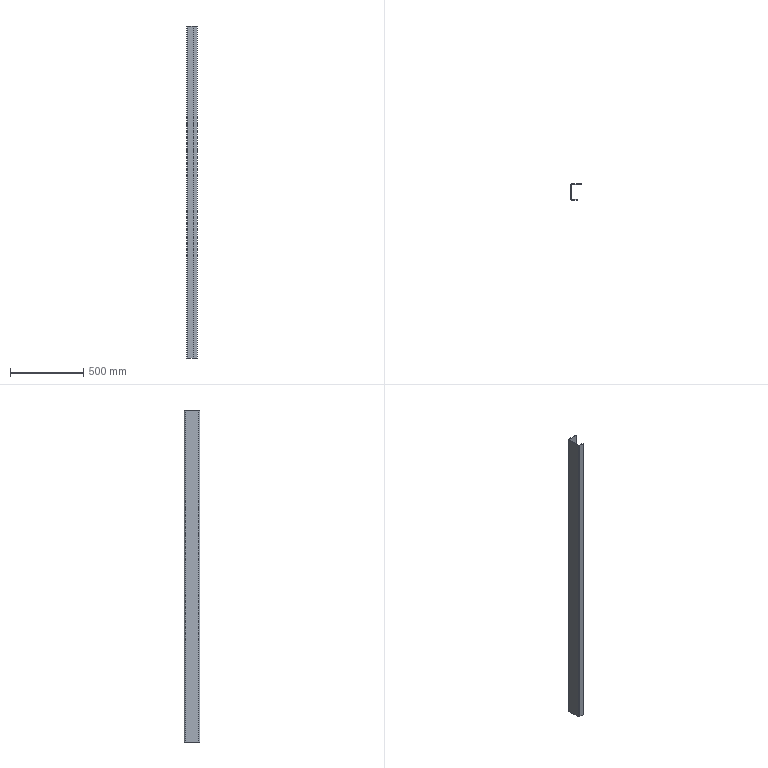Part | STEP file | 750038121 | 1 solid | 14 faces | box 75 x 108 x 2272 mm | volume 1952553 mm3 | plane 10 | cylinder 4 | commonest cylinder face diameters 8 x2 16 x2
STEP:
#1=CARTESIAN_POINT('',(0.,8.,0.));
#2=VERTEX_POINT('',#1);
#3=CARTESIAN_POINT('',(0.,100.,0.));
#4=VERTEX_POINT('',#3);
#5=CARTESIAN_POINT('',(0.,0.,0.));
#6=DIRECTION('',(0.,1.,0.));
#7=VECTOR('',#6,1000.);
#8=LINE('',#5,#7);
#9=EDGE_CURVE('',#2,#4,#8,.T.);
#10=ORIENTED_EDGE('',*,*,#9,.T.);
#11=CARTESIAN_POINT('',(0.,100.,-2272.));
#12=VERTEX_POINT('',#11);
#13=CARTESIAN_POINT('',(0.,100.,0.));
#14=DIRECTION('',(0.,0.,-1.));
#15=VECTOR('',#14,1000.);
#16=LINE('',#13,#15);
#17=EDGE_CURVE('',#4,#12,#16,.T.);
#18=ORIENTED_EDGE('',*,*,#17,.T.);
#19=CARTESIAN_POINT('',(0.,8.,-2272.));
#20=VERTEX_POINT('',#19);
#21=CARTESIAN_POINT('',(0.,0.,-2272.));
#22=DIRECTION('',(0.,-1.,0.));
#23=VECTOR('',#22,1000.);
#24=LINE('',#21,#23);
#25=EDGE_CURVE('',#12,#20,#24,.T.);
#26=ORIENTED_EDGE('',*,*,#25,.T.);
#27=CARTESIAN_POINT('',(0.,8.,0.));
#28=DIRECTION('',(0.,0.,1.));
#29=VECTOR('',#28,1000.);
#30=LINE('',#27,#29);
#31=EDGE_CURVE('',#20,#2,#30,.T.);
#32=ORIENTED_EDGE('',*,*,#31,.T.);
#33=EDGE_LOOP('',(#10,#18,#26,#32));
#34=FACE_OUTER_BOUND('',#33,.T.);
#35=CARTESIAN_POINT('',(0.,0.,0.));
#36=DIRECTION('',(-1.,0.,0.));
#37=DIRECTION('',(0.,0.,1.));
#38=AXIS2_PLACEMENT_3D('',#35,#36,#37);
#39=PLANE('',#38);
#40=ADVANCED_FACE('',(#34),#39,.T.);
#41=CARTESIAN_POINT('',(8.,108.,0.));
#42=VERTEX_POINT('',#41);
#43=CARTESIAN_POINT('',(8.,100.,0.));
#44=DIRECTION('',(0.,0.,-1.));
#45=DIRECTION('',(-1.,0.,0.));
#46=AXIS2_PLACEMENT_3D('',#43,#44,#45);
#47=CIRCLE('',#46,8.);
#48=EDGE_CURVE('',#4,#42,#47,.T.);
#49=ORIENTED_EDGE('',*,*,#48,.T.);
#50=CARTESIAN_POINT('',(8.,108.,-2272.));
#51=VERTEX_POINT('',#50);
#52=CARTESIAN_POINT('',(8.,108.,0.));
#53=DIRECTION('',(0.,0.,-1.));
#54=VECTOR('',#53,1000.);
#55=LINE('',#52,#54);
#56=EDGE_CURVE('',#42,#51,#55,.T.);
#57=ORIENTED_EDGE('',*,*,#56,.T.);
#58=CARTESIAN_POINT('',(8.,100.,-2272.));
#59=DIRECTION('',(0.,0.,1.));
#60=DIRECTION('',(-1.,0.,0.));
#61=AXIS2_PLACEMENT_3D('',#58,#59,#60);
#62=CIRCLE('',#61,8.);
#63=EDGE_CURVE('',#51,#12,#62,.T.);
#64=ORIENTED_EDGE('',*,*,#63,.T.);
#65=ORIENTED_EDGE('',*,*,#17,.F.);
#66=EDGE_LOOP('',(#49,#57,#64,#65));
#67=FACE_OUTER_BOUND('',#66,.T.);
#68=CARTESIAN_POINT('',(8.,100.,0.));
#69=DIRECTION('',(0.,0.,-1.));
#70=DIRECTION('',(-1.,0.,0.));
#71=AXIS2_PLACEMENT_3D('',#68,#69,#70);
#72=CYLINDRICAL_SURFACE('',#71,8.);
#73=ADVANCED_FACE('',(#67),#72,.T.);
#74=CARTESIAN_POINT('',(8.,104.,0.));
#75=VERTEX_POINT('',#74);
#76=CARTESIAN_POINT('',(75.,104.,0.));
#77=VERTEX_POINT('',#76);
#78=CARTESIAN_POINT('',(0.,104.,0.));
#79=DIRECTION('',(1.,0.,0.));
#80=VECTOR('',#79,1000.);
#81=LINE('',#78,#80);
#82=EDGE_CURVE('',#75,#77,#81,.T.);
#83=ORIENTED_EDGE('',*,*,#82,.T.);
#84=CARTESIAN_POINT('',(75.,108.,0.));
#85=VERTEX_POINT('',#84);
#86=CARTESIAN_POINT('',(75.,108.,0.));
#87=DIRECTION('',(0.,1.,0.));
#88=VECTOR('',#87,1000.);
#89=LINE('',#86,#88);
#90=EDGE_CURVE('',#77,#85,#89,.T.);
#91=ORIENTED_EDGE('',*,*,#90,.T.);
#92=CARTESIAN_POINT('',(0.,108.,0.));
#93=DIRECTION('',(-1.,0.,0.));
#94=VECTOR('',#93,1000.);
#95=LINE('',#92,#94);
#96=EDGE_CURVE('',#85,#42,#95,.T.);
#97=ORIENTED_EDGE('',*,*,#96,.T.);
#98=ORIENTED_EDGE('',*,*,#48,.F.);
#99=ORIENTED_EDGE('',*,*,#9,.F.);
#100=CARTESIAN_POINT('',(8.,0.,0.));
#101=VERTEX_POINT('',#100);
#102=CARTESIAN_POINT('',(8.,8.,0.));
#103=DIRECTION('',(0.,0.,1.));
#104=DIRECTION('',(-1.,0.,0.));
#105=AXIS2_PLACEMENT_3D('',#102,#103,#104);
#106=CIRCLE('',#105,8.);
#107=EDGE_CURVE('',#2,#101,#106,.T.);
#108=ORIENTED_EDGE('',*,*,#107,.T.);
#109=CARTESIAN_POINT('',(45.,0.,0.));
#110=VERTEX_POINT('',#109);
#111=CARTESIAN_POINT('',(0.,0.,0.));
#112=DIRECTION('',(1.,0.,0.));
#113=VECTOR('',#112,1000.);
#114=LINE('',#111,#113);
#115=EDGE_CURVE('',#101,#110,#114,.T.);
#116=ORIENTED_EDGE('',*,*,#115,.T.);
#117=CARTESIAN_POINT('',(45.,4.,0.));
#118=VERTEX_POINT('',#117);
#119=CARTESIAN_POINT('',(45.,108.,0.));
#120=DIRECTION('',(0.,1.,0.));
#121=VECTOR('',#120,1000.);
#122=LINE('',#119,#121);
#123=EDGE_CURVE('',#110,#118,#122,.T.);
#124=ORIENTED_EDGE('',*,*,#123,.T.);
#125=CARTESIAN_POINT('',(8.,4.,0.));
#126=VERTEX_POINT('',#125);
#127=CARTESIAN_POINT('',(0.,4.,0.));
#128=DIRECTION('',(-1.,0.,0.));
#129=VECTOR('',#128,1000.);
#130=LINE('',#127,#129);
#131=EDGE_CURVE('',#118,#126,#130,.T.);
#132=ORIENTED_EDGE('',*,*,#131,.T.);
#133=CARTESIAN_POINT('',(4.,8.,0.));
#134=VERTEX_POINT('',#133);
#135=CARTESIAN_POINT('',(8.,8.,0.));
#136=DIRECTION('',(0.,0.,-1.));
#137=DIRECTION('',(-1.,0.,0.));
#138=AXIS2_PLACEMENT_3D('',#135,#136,#137);
#139=CIRCLE('',#138,4.);
#140=EDGE_CURVE('',#126,#134,#139,.T.);
#141=ORIENTED_EDGE('',*,*,#140,.T.);
#142=CARTESIAN_POINT('',(4.,100.,0.));
#143=VERTEX_POINT('',#142);
#144=CARTESIAN_POINT('',(4.,108.,0.));
#145=DIRECTION('',(0.,1.,0.));
#146=VECTOR('',#145,1000.);
#147=LINE('',#144,#146);
#148=EDGE_CURVE('',#134,#143,#147,.T.);
#149=ORIENTED_EDGE('',*,*,#148,.T.);
#150=CARTESIAN_POINT('',(8.,100.,0.));
#151=DIRECTION('',(0.,0.,-1.));
#152=DIRECTION('',(-1.,0.,0.));
#153=AXIS2_PLACEMENT_3D('',#150,#151,#152);
#154=CIRCLE('',#153,4.);
#155=EDGE_CURVE('',#143,#75,#154,.T.);
#156=ORIENTED_EDGE('',*,*,#155,.T.);
#157=EDGE_LOOP('',(#83,#91,#97,#98,#99,#108,#116,#124,#132,#141,#149,#156));
#158=FACE_OUTER_BOUND('',#157,.T.);
#159=CARTESIAN_POINT('',(0.,108.,0.));
#160=DIRECTION('',(0.,0.,1.));
#161=DIRECTION('',(1.,0.,0.));
#162=AXIS2_PLACEMENT_3D('',#159,#160,#161);
#163=PLANE('',#162);
#164=ADVANCED_FACE('',(#158),#163,.T.);
#165=ORIENTED_EDGE('',*,*,#107,.F.);
#166=ORIENTED_EDGE('',*,*,#31,.F.);
#167=CARTESIAN_POINT('',(8.,0.,-2272.));
#168=VERTEX_POINT('',#167);
#169=CARTESIAN_POINT('',(8.,8.,-2272.));
#170=DIRECTION('',(0.,0.,1.));
#171=DIRECTION('',(-1.,0.,0.));
#172=AXIS2_PLACEMENT_3D('',#169,#170,#171);
#173=CIRCLE('',#172,8.);
#174=EDGE_CURVE('',#20,#168,#173,.T.);
#175=ORIENTED_EDGE('',*,*,#174,.T.);
#176=CARTESIAN_POINT('',(8.,0.,0.));
#177=DIRECTION('',(0.,0.,1.));
#178=VECTOR('',#177,1000.);
#179=LINE('',#176,#178);
#180=EDGE_CURVE('',#168,#101,#179,.T.);
#181=ORIENTED_EDGE('',*,*,#180,.T.);
#182=EDGE_LOOP('',(#165,#166,#175,#181));
#183=FACE_OUTER_BOUND('',#182,.T.);
#184=CARTESIAN_POINT('',(8.,8.,0.));
#185=DIRECTION('',(0.,0.,-1.));
#186=DIRECTION('',(-1.,0.,0.));
#187=AXIS2_PLACEMENT_3D('',#184,#185,#186);
#188=CYLINDRICAL_SURFACE('',#187,8.);
#189=ADVANCED_FACE('',(#183),#188,.T.);
#190=ORIENTED_EDGE('',*,*,#174,.F.);
#191=ORIENTED_EDGE('',*,*,#25,.F.);
#192=ORIENTED_EDGE('',*,*,#63,.F.);
#193=CARTESIAN_POINT('',(75.,108.,-2272.));
#194=VERTEX_POINT('',#193);
#195=CARTESIAN_POINT('',(45.,108.,-2272.));
#196=DIRECTION('',(-1.,0.,0.));
#197=VECTOR('',#196,1000.);
#198=LINE('',#195,#197);
#199=EDGE_CURVE('',#194,#51,#198,.T.);
#200=ORIENTED_EDGE('',*,*,#199,.F.);
#201=CARTESIAN_POINT('',(75.,104.,-2272.));
#202=VERTEX_POINT('',#201);
#203=CARTESIAN_POINT('',(75.,0.,-2272.));
#204=DIRECTION('',(0.,1.,0.));
#205=VECTOR('',#204,1000.);
#206=LINE('',#203,#205);
#207=EDGE_CURVE('',#202,#194,#206,.T.);
#208=ORIENTED_EDGE('',*,*,#207,.F.);
#209=CARTESIAN_POINT('',(8.,104.,-2272.));
#210=VERTEX_POINT('',#209);
#211=CARTESIAN_POINT('',(45.,104.,-2272.));
#212=DIRECTION('',(1.,0.,0.));
#213=VECTOR('',#212,1000.);
#214=LINE('',#211,#213);
#215=EDGE_CURVE('',#210,#202,#214,.T.);
#216=ORIENTED_EDGE('',*,*,#215,.F.);
#217=CARTESIAN_POINT('',(4.,100.,-2272.));
#218=VERTEX_POINT('',#217);
#219=CARTESIAN_POINT('',(8.,100.,-2272.));
#220=DIRECTION('',(0.,0.,-1.));
#221=DIRECTION('',(-1.,0.,0.));
#222=AXIS2_PLACEMENT_3D('',#219,#220,#221);
#223=CIRCLE('',#222,4.);
#224=EDGE_CURVE('',#218,#210,#223,.T.);
#225=ORIENTED_EDGE('',*,*,#224,.F.);
#226=CARTESIAN_POINT('',(4.,8.,-2272.));
#227=VERTEX_POINT('',#226);
#228=CARTESIAN_POINT('',(4.,0.,-2272.));
#229=DIRECTION('',(0.,1.,0.));
#230=VECTOR('',#229,1000.);
#231=LINE('',#228,#230);
#232=EDGE_CURVE('',#227,#218,#231,.T.);
#233=ORIENTED_EDGE('',*,*,#232,.F.);
#234=CARTESIAN_POINT('',(8.,4.,-2272.));
#235=VERTEX_POINT('',#234);
#236=CARTESIAN_POINT('',(8.,8.,-2272.));
#237=DIRECTION('',(0.,0.,-1.));
#238=DIRECTION('',(-1.,0.,0.));
#239=AXIS2_PLACEMENT_3D('',#236,#237,#238);
#240=CIRCLE('',#239,4.);
#241=EDGE_CURVE('',#235,#227,#240,.T.);
#242=ORIENTED_EDGE('',*,*,#241,.F.);
#243=CARTESIAN_POINT('',(45.,4.,-2272.));
#244=VERTEX_POINT('',#243);
#245=CARTESIAN_POINT('',(45.,4.,-2272.));
#246=DIRECTION('',(-1.,0.,0.));
#247=VECTOR('',#246,1000.);
#248=LINE('',#245,#247);
#249=EDGE_CURVE('',#244,#235,#248,.T.);
#250=ORIENTED_EDGE('',*,*,#249,.F.);
#251=CARTESIAN_POINT('',(45.,0.,-2272.));
#252=VERTEX_POINT('',#251);
#253=CARTESIAN_POINT('',(45.,0.,-2272.));
#254=DIRECTION('',(0.,1.,0.));
#255=VECTOR('',#254,1000.);
#256=LINE('',#253,#255);
#257=EDGE_CURVE('',#252,#244,#256,.T.);
#258=ORIENTED_EDGE('',*,*,#257,.F.);
#259=CARTESIAN_POINT('',(45.,0.,-2272.));
#260=DIRECTION('',(1.,0.,0.));
#261=VECTOR('',#260,1000.);
#262=LINE('',#259,#261);
#263=EDGE_CURVE('',#168,#252,#262,.T.);
#264=ORIENTED_EDGE('',*,*,#263,.F.);
#265=EDGE_LOOP('',(#190,#191,#192,#200,#208,#216,#225,#233,#242,#250,#258,#264));
#266=FACE_OUTER_BOUND('',#265,.T.);
#267=CARTESIAN_POINT('',(45.,0.,-2272.));
#268=DIRECTION('',(0.,0.,1.));
#269=DIRECTION('',(1.,0.,0.));
#270=AXIS2_PLACEMENT_3D('',#267,#268,#269);
#271=PLANE('',#270);
#272=ADVANCED_FACE('',(#266),#271,.F.);
#273=ORIENTED_EDGE('',*,*,#96,.F.);
#274=CARTESIAN_POINT('',(75.,108.,0.));
#275=DIRECTION('',(0.,0.,-1.));
#276=VECTOR('',#275,1000.);
#277=LINE('',#274,#276);
#278=EDGE_CURVE('',#85,#194,#277,.T.);
#279=ORIENTED_EDGE('',*,*,#278,.T.);
#280=ORIENTED_EDGE('',*,*,#199,.T.);
#281=ORIENTED_EDGE('',*,*,#56,.F.);
#282=EDGE_LOOP('',(#273,#279,#280,#281));
#283=FACE_OUTER_BOUND('',#282,.T.);
#284=CARTESIAN_POINT('',(0.,108.,0.));
#285=DIRECTION('',(0.,1.,0.));
#286=DIRECTION('',(0.,0.,1.));
#287=AXIS2_PLACEMENT_3D('',#284,#285,#286);
#288=PLANE('',#287);
#289=ADVANCED_FACE('',(#283),#288,.T.);
#290=ORIENTED_EDGE('',*,*,#207,.T.);
#291=ORIENTED_EDGE('',*,*,#278,.F.);
#292=ORIENTED_EDGE('',*,*,#90,.F.);
#293=CARTESIAN_POINT('',(75.,104.,0.));
#294=DIRECTION('',(0.,0.,-1.));
#295=VECTOR('',#294,1000.);
#296=LINE('',#293,#295);
#297=EDGE_CURVE('',#77,#202,#296,.T.);
#298=ORIENTED_EDGE('',*,*,#297,.T.);
#299=EDGE_LOOP('',(#290,#291,#292,#298));
#300=FACE_OUTER_BOUND('',#299,.T.);
#301=CARTESIAN_POINT('',(75.,108.,0.));
#302=DIRECTION('',(1.,0.,0.));
#303=DIRECTION('',(0.,0.,-1.));
#304=AXIS2_PLACEMENT_3D('',#301,#302,#303);
#305=PLANE('',#304);
#306=ADVANCED_FACE('',(#300),#305,.T.);
#307=ORIENTED_EDGE('',*,*,#297,.F.);
#308=ORIENTED_EDGE('',*,*,#82,.F.);
#309=CARTESIAN_POINT('',(8.,104.,0.));
#310=DIRECTION('',(0.,0.,1.));
#311=VECTOR('',#310,1000.);
#312=LINE('',#309,#311);
#313=EDGE_CURVE('',#210,#75,#312,.T.);
#314=ORIENTED_EDGE('',*,*,#313,.F.);
#315=ORIENTED_EDGE('',*,*,#215,.T.);
#316=EDGE_LOOP('',(#307,#308,#314,#315));
#317=FACE_OUTER_BOUND('',#316,.T.);
#318=CARTESIAN_POINT('',(0.,104.,0.));
#319=DIRECTION('',(0.,1.,0.));
#320=DIRECTION('',(0.,0.,1.));
#321=AXIS2_PLACEMENT_3D('',#318,#319,#320);
#322=PLANE('',#321);
#323=ADVANCED_FACE('',(#317),#322,.F.);
#324=ORIENTED_EDGE('',*,*,#313,.T.);
#325=ORIENTED_EDGE('',*,*,#155,.F.);
#326=CARTESIAN_POINT('',(4.,100.,0.));
#327=DIRECTION('',(0.,0.,1.));
#328=VECTOR('',#327,1000.);
#329=LINE('',#326,#328);
#330=EDGE_CURVE('',#218,#143,#329,.T.);
#331=ORIENTED_EDGE('',*,*,#330,.F.);
#332=ORIENTED_EDGE('',*,*,#224,.T.);
#333=EDGE_LOOP('',(#324,#325,#331,#332));
#334=FACE_OUTER_BOUND('',#333,.T.);
#335=CARTESIAN_POINT('',(8.,100.,0.));
#336=DIRECTION('',(0.,0.,-1.));
#337=DIRECTION('',(-1.,0.,0.));
#338=AXIS2_PLACEMENT_3D('',#335,#336,#337);
#339=CYLINDRICAL_SURFACE('',#338,4.);
#340=ADVANCED_FACE('',(#334),#339,.F.);
#341=ORIENTED_EDGE('',*,*,#330,.T.);
#342=ORIENTED_EDGE('',*,*,#148,.F.);
#343=CARTESIAN_POINT('',(4.,8.,0.));
#344=DIRECTION('',(0.,0.,1.));
#345=VECTOR('',#344,1000.);
#346=LINE('',#343,#345);
#347=EDGE_CURVE('',#227,#134,#346,.T.);
#348=ORIENTED_EDGE('',*,*,#347,.F.);
#349=ORIENTED_EDGE('',*,*,#232,.T.);
#350=EDGE_LOOP('',(#341,#342,#348,#349));
#351=FACE_OUTER_BOUND('',#350,.T.);
#352=CARTESIAN_POINT('',(4.,0.,0.));
#353=DIRECTION('',(-1.,0.,0.));
#354=DIRECTION('',(0.,0.,1.));
#355=AXIS2_PLACEMENT_3D('',#352,#353,#354);
#356=PLANE('',#355);
#357=ADVANCED_FACE('',(#351),#356,.F.);
#358=ORIENTED_EDGE('',*,*,#347,.T.);
#359=ORIENTED_EDGE('',*,*,#140,.F.);
#360=CARTESIAN_POINT('',(8.,4.,0.));
#361=DIRECTION('',(0.,0.,1.));
#362=VECTOR('',#361,1000.);
#363=LINE('',#360,#362);
#364=EDGE_CURVE('',#235,#126,#363,.T.);
#365=ORIENTED_EDGE('',*,*,#364,.F.);
#366=ORIENTED_EDGE('',*,*,#241,.T.);
#367=EDGE_LOOP('',(#358,#359,#365,#366));
#368=FACE_OUTER_BOUND('',#367,.T.);
#369=CARTESIAN_POINT('',(8.,8.,0.));
#370=DIRECTION('',(0.,0.,-1.));
#371=DIRECTION('',(-1.,0.,0.));
#372=AXIS2_PLACEMENT_3D('',#369,#370,#371);
#373=CYLINDRICAL_SURFACE('',#372,4.);
#374=ADVANCED_FACE('',(#368),#373,.F.);
#375=ORIENTED_EDGE('',*,*,#364,.T.);
#376=ORIENTED_EDGE('',*,*,#131,.F.);
#377=CARTESIAN_POINT('',(45.,4.,0.));
#378=DIRECTION('',(0.,0.,1.));
#379=VECTOR('',#378,1000.);
#380=LINE('',#377,#379);
#381=EDGE_CURVE('',#244,#118,#380,.T.);
#382=ORIENTED_EDGE('',*,*,#381,.F.);
#383=ORIENTED_EDGE('',*,*,#249,.T.);
#384=EDGE_LOOP('',(#375,#376,#382,#383));
#385=FACE_OUTER_BOUND('',#384,.T.);
#386=CARTESIAN_POINT('',(45.,4.,0.));
#387=DIRECTION('',(0.,-1.,0.));
#388=DIRECTION('',(0.,0.,-1.));
#389=AXIS2_PLACEMENT_3D('',#386,#387,#388);
#390=PLANE('',#389);
#391=ADVANCED_FACE('',(#385),#390,.F.);
#392=ORIENTED_EDGE('',*,*,#123,.F.);
#393=CARTESIAN_POINT('',(45.,0.,0.));
#394=DIRECTION('',(0.,0.,1.));
#395=VECTOR('',#394,1000.);
#396=LINE('',#393,#395);
#397=EDGE_CURVE('',#252,#110,#396,.T.);
#398=ORIENTED_EDGE('',*,*,#397,.F.);
#399=ORIENTED_EDGE('',*,*,#257,.T.);
#400=ORIENTED_EDGE('',*,*,#381,.T.);
#401=EDGE_LOOP('',(#392,#398,#399,#400));
#402=FACE_OUTER_BOUND('',#401,.T.);
#403=CARTESIAN_POINT('',(45.,0.,0.));
#404=DIRECTION('',(-1.,0.,0.));
#405=DIRECTION('',(0.,0.,1.));
#406=AXIS2_PLACEMENT_3D('',#403,#404,#405);
#407=PLANE('',#406);
#408=ADVANCED_FACE('',(#402),#407,.F.);
#409=ORIENTED_EDGE('',*,*,#115,.F.);
#410=ORIENTED_EDGE('',*,*,#180,.F.);
#411=ORIENTED_EDGE('',*,*,#263,.T.);
#412=ORIENTED_EDGE('',*,*,#397,.T.);
#413=EDGE_LOOP('',(#409,#410,#411,#412));
#414=FACE_OUTER_BOUND('',#413,.T.);
#415=CARTESIAN_POINT('',(45.,0.,0.));
#416=DIRECTION('',(0.,-1.,0.));
#417=DIRECTION('',(0.,0.,-1.));
#418=AXIS2_PLACEMENT_3D('',#415,#416,#417);
#419=PLANE('',#418);
#420=ADVANCED_FACE('',(#414),#419,.T.);
#421=CLOSED_SHELL('',(#40,#73,#164,#189,#272,#289,#306,#323,#340,#357,#374,#391,#408,#420));
#422=MANIFOLD_SOLID_BREP('',#421);
#423=CARTESIAN_POINT('',(0.,0.,0.));
#424=DIRECTION('',(0.,0.,1.));
#425=DIRECTION('',(1.,0.,0.));
#426=AXIS2_PLACEMENT_3D('',#423,#424,#425);
#427=(LENGTH_UNIT()NAMED_UNIT(*)SI_UNIT(.MILLI.,.METRE.));
#428=UNCERTAINTY_MEASURE_WITH_UNIT(LENGTH_MEASURE(0.00001),#427,'','');
#429=(NAMED_UNIT(*)PLANE_ANGLE_UNIT()SI_UNIT($,.RADIAN.));
#430=(NAMED_UNIT(*)SI_UNIT($,.STERADIAN.)SOLID_ANGLE_UNIT());
#431=(GEOMETRIC_REPRESENTATION_CONTEXT(3)GLOBAL_UNCERTAINTY_ASSIGNED_CONTEXT((#428))GLOBAL_UNIT_ASSIGNED_CONTEXT((#427,#429,#430))REPRESENTATION_CONTEXT('',''));
#432=ADVANCED_BREP_SHAPE_REPRESENTATION('',(#422,#426),#431);